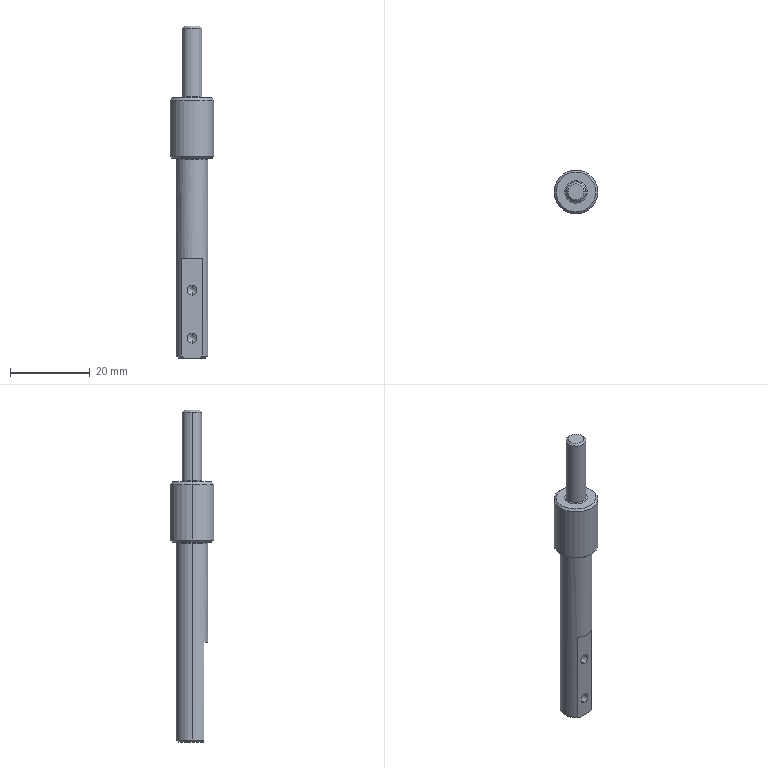Part | STEP file | Conductive post-market | 1 solid | 33 faces | box 11 x 11 x 83 mm | volume 4143 mm3 | cone 13 | cylinder 10 | plane 6 | spline 4 | commonest cylinder face diameters 2.5 x4 5 x2 8 x2 11 x2